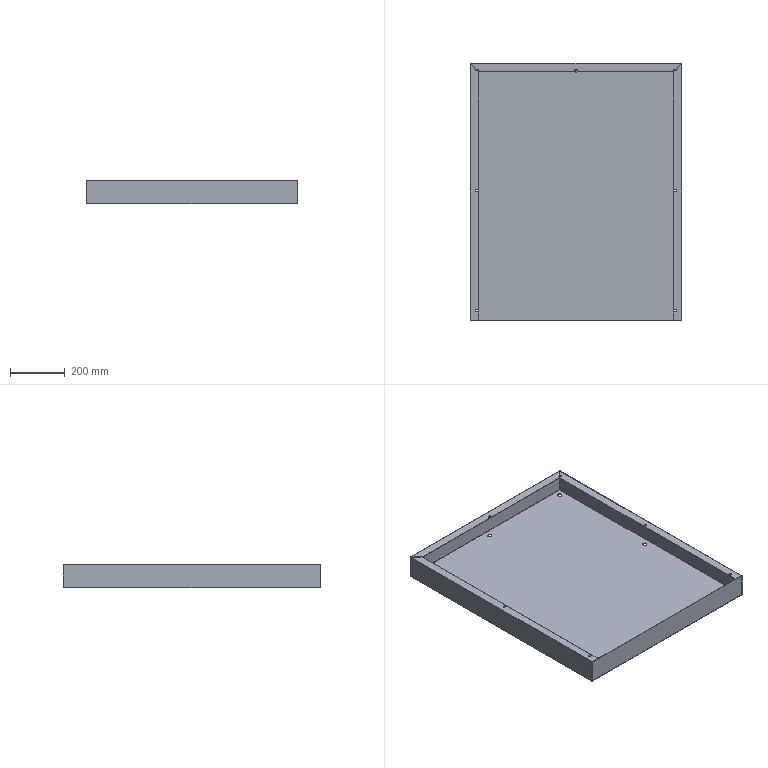Part | SolidWorks | features BaseBody 1 | 1 solid | 132 faces | box 776 x 944 x 86.5 mm | volume 1648928 mm3 | plane 76 | cylinder 52 | spline 4 | commonest cylinder face diameters 6.5 x24 15 x14 0.4 x7 3.4 x7